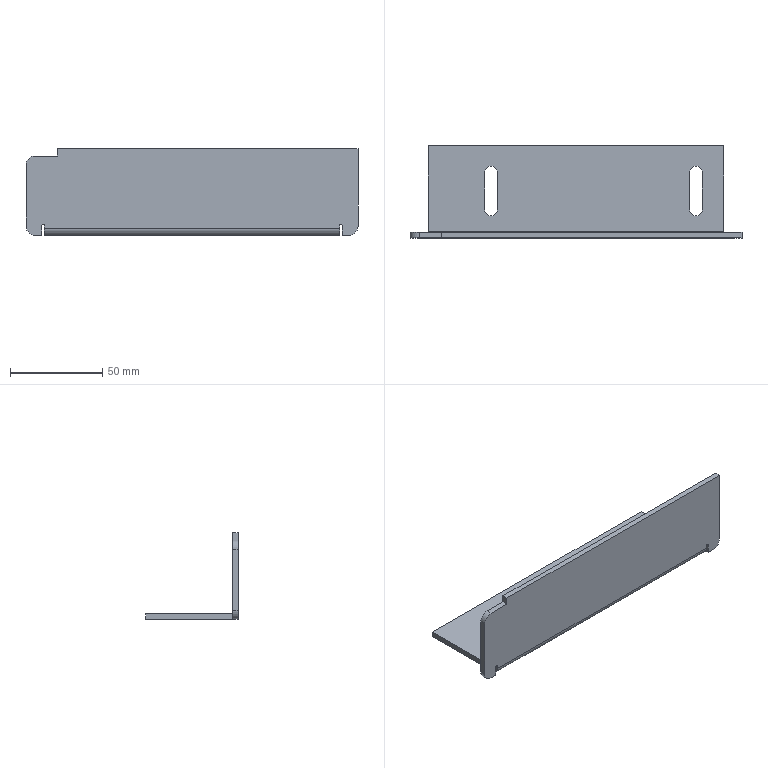Part | STEP file | PN_0049_cover_default_machined_ | 1 solid | 31 faces | box 180 x 50 x 47 mm | volume 46104 mm3 | plane 20 | cylinder 11 | commonest cylinder face diameters 7 x4 10 x3 1.5 x2 1.473 x1 7.473 x1